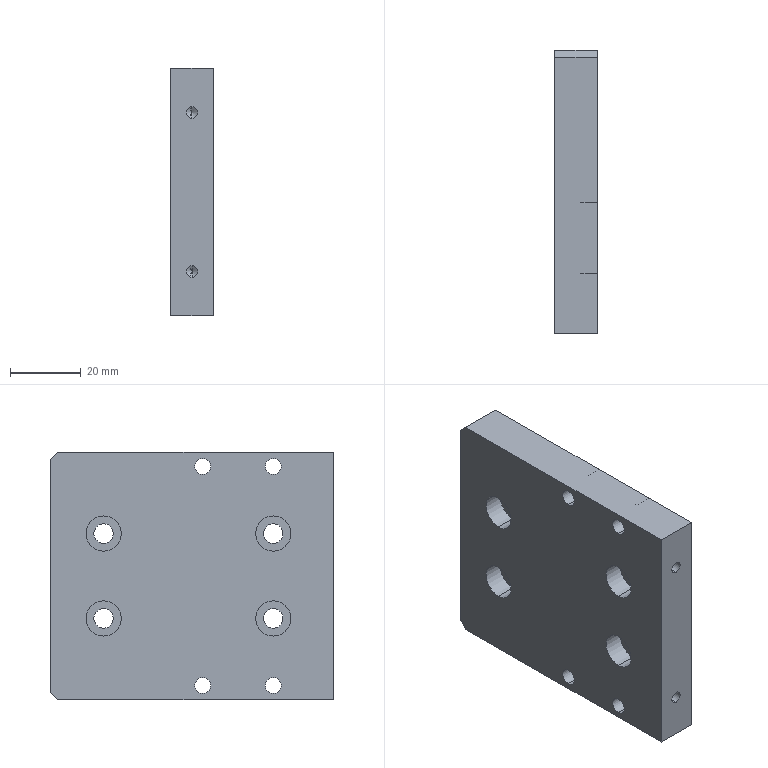Part | SolidWorks | features HoleWzd 3, Chamfer 1, Extrusion 1 | 1 solid | 56 faces | box 12 x 80 x 70 mm | volume 63301 mm3 | cylinder 36 | plane 16 | cone 4 | commonest cylinder face diameters 4.5 x8 5.5 x8 7.5 x8 10 x8 3.3 x4